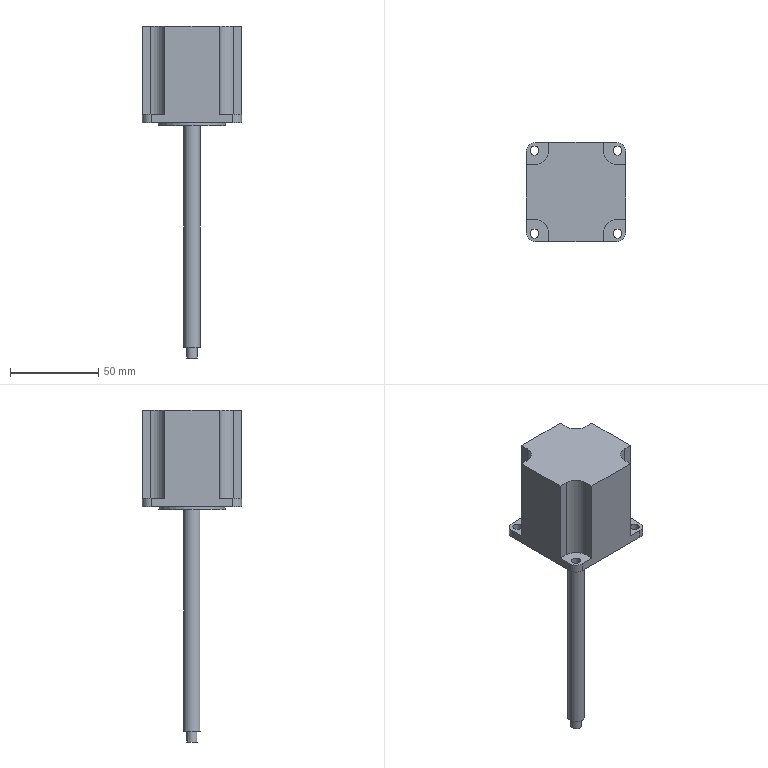Part | NX | features DATUM_CSYS 7, EXTRUDE 6, SKETCH 6, BLEND 1, DISTANCE MEASUREMENT 1, SYMBOLIC_THREAD 1 | 1 solid | 36 faces | box 56.4 x 56.4 x 188.6 mm | volume 156156 mm3 | plane 21 | cylinder 15 | commonest cylinder face diameters 5.1 x4 10 x4 16 x4 6 x1 9.525 x1 38.1 x1
STEP:
#1=CARTESIAN_POINT('',(-23.2,-28.2,4.8));
#2=VERTEX_POINT('',#1);
#3=CARTESIAN_POINT('',(-15.57,-28.2,4.8));
#4=VERTEX_POINT('',#3);
#5=CARTESIAN_POINT('',(-28.2,-28.2,4.8));
#6=DIRECTION('',(1.,0.,0.));
#7=VECTOR('',#6,1000.);
#8=LINE('',#5,#7);
#9=EDGE_CURVE('',#2,#4,#8,.T.);
#10=ORIENTED_EDGE('',*,*,#9,.F.);
#11=CARTESIAN_POINT('',(-23.2,-28.2,0.));
#12=VERTEX_POINT('',#11);
#13=CARTESIAN_POINT('',(-23.2,-28.2,55.));
#14=DIRECTION('',(0.,0.,-1.));
#15=VECTOR('',#14,1000.);
#16=LINE('',#13,#15);
#17=EDGE_CURVE('',#2,#12,#16,.T.);
#18=ORIENTED_EDGE('',*,*,#17,.T.);
#19=CARTESIAN_POINT('',(23.2,-28.2,0.));
#20=VERTEX_POINT('',#19);
#21=CARTESIAN_POINT('',(-28.2,-28.2,0.));
#22=DIRECTION('',(1.,0.,0.));
#23=VECTOR('',#22,1000.);
#24=LINE('',#21,#23);
#25=EDGE_CURVE('',#12,#20,#24,.T.);
#26=ORIENTED_EDGE('',*,*,#25,.T.);
#27=CARTESIAN_POINT('',(23.2,-28.2,4.8));
#28=VERTEX_POINT('',#27);
#29=CARTESIAN_POINT('',(23.2,-28.2,55.));
#30=DIRECTION('',(0.,0.,-1.));
#31=VECTOR('',#30,1000.);
#32=LINE('',#29,#31);
#33=EDGE_CURVE('',#20,#28,#32,.F.);
#34=ORIENTED_EDGE('',*,*,#33,.T.);
#35=CARTESIAN_POINT('',(15.57,-28.2,4.8));
#36=VERTEX_POINT('',#35);
#37=CARTESIAN_POINT('',(15.57,-28.2,4.8));
#38=DIRECTION('',(1.,0.,0.));
#39=VECTOR('',#38,1000.);
#40=LINE('',#37,#39);
#41=EDGE_CURVE('',#36,#28,#40,.T.);
#42=ORIENTED_EDGE('',*,*,#41,.F.);
#43=CARTESIAN_POINT('',(15.57,-28.2,55.));
#44=VERTEX_POINT('',#43);
#45=CARTESIAN_POINT('',(15.57,-28.2,4.8));
#46=DIRECTION('',(0.,0.,1.));
#47=VECTOR('',#46,1000.);
#48=LINE('',#45,#47);
#49=EDGE_CURVE('',#36,#44,#48,.T.);
#50=ORIENTED_EDGE('',*,*,#49,.T.);
#51=CARTESIAN_POINT('',(-15.57,-28.2,55.));
#52=VERTEX_POINT('',#51);
#53=CARTESIAN_POINT('',(-28.2,-28.2,55.));
#54=DIRECTION('',(1.,0.,0.));
#55=VECTOR('',#54,1000.);
#56=LINE('',#53,#55);
#57=EDGE_CURVE('',#52,#44,#56,.T.);
#58=ORIENTED_EDGE('',*,*,#57,.F.);
#59=CARTESIAN_POINT('',(-15.57,-28.2,4.8));
#60=DIRECTION('',(0.,0.,1.));
#61=VECTOR('',#60,1000.);
#62=LINE('',#59,#61);
#63=EDGE_CURVE('',#4,#52,#62,.T.);
#64=ORIENTED_EDGE('',*,*,#63,.F.);
#65=EDGE_LOOP('',(#10,#18,#26,#34,#42,#50,#58,#64));
#66=FACE_BOUND('',#65,.T.);
#67=CARTESIAN_POINT('',(-28.2,-28.2,55.));
#68=DIRECTION('',(0.,1.,0.));
#69=DIRECTION('',(0.,0.,1.));
#70=AXIS2_PLACEMENT_3D('',#67,#68,#69);
#71=PLANE('',#70);
#72=ADVANCED_FACE('',(#66),#71,.F.);
#73=CARTESIAN_POINT('',(-21.02,-23.57,0.));
#74=VERTEX_POINT('',#73);
#75=CARTESIAN_POINT('',(-23.57,-23.57,0.));
#76=DIRECTION('',(0.,0.,1.));
#77=DIRECTION('',(1.,0.,0.));
#78=AXIS2_PLACEMENT_3D('',#75,#76,#77);
#79=CIRCLE('',#78,2.55);
#80=EDGE_CURVE('',#74,#74,#79,.F.);
#81=ORIENTED_EDGE('',*,*,#80,.T.);
#82=EDGE_LOOP('',(#81));
#83=FACE_BOUND('',#82,.T.);
#84=CARTESIAN_POINT('',(-21.02,-23.57,4.8));
#85=VERTEX_POINT('',#84);
#86=CARTESIAN_POINT('',(-23.57,-23.57,4.8));
#87=DIRECTION('',(0.,0.,1.));
#88=DIRECTION('',(1.,0.,0.));
#89=AXIS2_PLACEMENT_3D('',#86,#87,#88);
#90=CIRCLE('',#89,2.55);
#91=EDGE_CURVE('',#85,#85,#90,.T.);
#92=ORIENTED_EDGE('',*,*,#91,.T.);
#93=EDGE_LOOP('',(#92));
#94=FACE_BOUND('',#93,.T.);
#95=CARTESIAN_POINT('',(-23.57,-23.57,-7.26));
#96=DIRECTION('',(0.,0.,1.));
#97=DIRECTION('',(1.,0.,0.));
#98=AXIS2_PLACEMENT_3D('',#95,#96,#97);
#99=CYLINDRICAL_SURFACE('',#98,2.55);
#100=ADVANCED_FACE('',(#83,#94),#99,.F.);
#101=CARTESIAN_POINT('',(-28.2,23.2,0.));
#102=VERTEX_POINT('',#101);
#103=CARTESIAN_POINT('',(-28.2,-23.2,0.));
#104=VERTEX_POINT('',#103);
#105=CARTESIAN_POINT('',(-28.2,28.2,0.));
#106=DIRECTION('',(0.,-1.,0.));
#107=VECTOR('',#106,1000.);
#108=LINE('',#105,#107);
#109=EDGE_CURVE('',#102,#104,#108,.T.);
#110=ORIENTED_EDGE('',*,*,#109,.T.);
#111=CARTESIAN_POINT('',(-28.2,-23.2,4.8));
#112=VERTEX_POINT('',#111);
#113=CARTESIAN_POINT('',(-28.2,-23.2,55.));
#114=DIRECTION('',(0.,0.,-1.));
#115=VECTOR('',#114,1000.);
#116=LINE('',#113,#115);
#117=EDGE_CURVE('',#104,#112,#116,.F.);
#118=ORIENTED_EDGE('',*,*,#117,.T.);
#119=CARTESIAN_POINT('',(-28.2,-15.57,4.8));
#120=VERTEX_POINT('',#119);
#121=CARTESIAN_POINT('',(-28.2,-15.57,4.8));
#122=DIRECTION('',(0.,-1.,0.));
#123=VECTOR('',#122,1000.);
#124=LINE('',#121,#123);
#125=EDGE_CURVE('',#120,#112,#124,.T.);
#126=ORIENTED_EDGE('',*,*,#125,.F.);
#127=CARTESIAN_POINT('',(-28.2,-15.57,55.));
#128=VERTEX_POINT('',#127);
#129=CARTESIAN_POINT('',(-28.2,-15.57,4.8));
#130=DIRECTION('',(0.,0.,1.));
#131=VECTOR('',#130,1000.);
#132=LINE('',#129,#131);
#133=EDGE_CURVE('',#120,#128,#132,.T.);
#134=ORIENTED_EDGE('',*,*,#133,.T.);
#135=CARTESIAN_POINT('',(-28.2,15.57,55.));
#136=VERTEX_POINT('',#135);
#137=CARTESIAN_POINT('',(-28.2,28.2,55.));
#138=DIRECTION('',(0.,-1.,0.));
#139=VECTOR('',#138,1000.);
#140=LINE('',#137,#139);
#141=EDGE_CURVE('',#136,#128,#140,.T.);
#142=ORIENTED_EDGE('',*,*,#141,.F.);
#143=CARTESIAN_POINT('',(-28.2,15.57,4.8));
#144=VERTEX_POINT('',#143);
#145=CARTESIAN_POINT('',(-28.2,15.57,4.8));
#146=DIRECTION('',(0.,0.,1.));
#147=VECTOR('',#146,1000.);
#148=LINE('',#145,#147);
#149=EDGE_CURVE('',#144,#136,#148,.T.);
#150=ORIENTED_EDGE('',*,*,#149,.F.);
#151=CARTESIAN_POINT('',(-28.2,23.2,4.8));
#152=VERTEX_POINT('',#151);
#153=CARTESIAN_POINT('',(-28.2,28.2,4.8));
#154=DIRECTION('',(0.,-1.,0.));
#155=VECTOR('',#154,1000.);
#156=LINE('',#153,#155);
#157=EDGE_CURVE('',#152,#144,#156,.T.);
#158=ORIENTED_EDGE('',*,*,#157,.F.);
#159=CARTESIAN_POINT('',(-28.2,23.2,55.));
#160=DIRECTION('',(0.,0.,-1.));
#161=VECTOR('',#160,1000.);
#162=LINE('',#159,#161);
#163=EDGE_CURVE('',#152,#102,#162,.T.);
#164=ORIENTED_EDGE('',*,*,#163,.T.);
#165=EDGE_LOOP('',(#110,#118,#126,#134,#142,#150,#158,#164));
#166=FACE_BOUND('',#165,.T.);
#167=CARTESIAN_POINT('',(-28.2,28.2,55.));
#168=DIRECTION('',(1.,0.,0.));
#169=DIRECTION('',(0.,0.,-1.));
#170=AXIS2_PLACEMENT_3D('',#167,#168,#169);
#171=PLANE('',#170);
#172=ADVANCED_FACE('',(#166),#171,.F.);
#173=CARTESIAN_POINT('',(28.2,-23.2,4.8));
#174=VERTEX_POINT('',#173);
#175=CARTESIAN_POINT('',(28.2,-15.57,4.8));
#176=VERTEX_POINT('',#175);
#177=CARTESIAN_POINT('',(28.2,-28.2,4.8));
#178=DIRECTION('',(0.,1.,0.));
#179=VECTOR('',#178,1000.);
#180=LINE('',#177,#179);
#181=EDGE_CURVE('',#174,#176,#180,.T.);
#182=ORIENTED_EDGE('',*,*,#181,.F.);
#183=CARTESIAN_POINT('',(28.2,-23.2,0.));
#184=VERTEX_POINT('',#183);
#185=CARTESIAN_POINT('',(28.2,-23.2,55.));
#186=DIRECTION('',(0.,0.,-1.));
#187=VECTOR('',#186,1000.);
#188=LINE('',#185,#187);
#189=EDGE_CURVE('',#174,#184,#188,.T.);
#190=ORIENTED_EDGE('',*,*,#189,.T.);
#191=CARTESIAN_POINT('',(28.2,23.2,0.));
#192=VERTEX_POINT('',#191);
#193=CARTESIAN_POINT('',(28.2,-28.2,0.));
#194=DIRECTION('',(0.,1.,0.));
#195=VECTOR('',#194,1000.);
#196=LINE('',#193,#195);
#197=EDGE_CURVE('',#184,#192,#196,.T.);
#198=ORIENTED_EDGE('',*,*,#197,.T.);
#199=CARTESIAN_POINT('',(28.2,23.2,4.8));
#200=VERTEX_POINT('',#199);
#201=CARTESIAN_POINT('',(28.2,23.2,55.));
#202=DIRECTION('',(0.,0.,-1.));
#203=VECTOR('',#202,1000.);
#204=LINE('',#201,#203);
#205=EDGE_CURVE('',#192,#200,#204,.F.);
#206=ORIENTED_EDGE('',*,*,#205,.T.);
#207=CARTESIAN_POINT('',(28.2,15.57,4.8));
#208=VERTEX_POINT('',#207);
#209=CARTESIAN_POINT('',(28.2,15.57,4.8));
#210=DIRECTION('',(0.,1.,0.));
#211=VECTOR('',#210,1000.);
#212=LINE('',#209,#211);
#213=EDGE_CURVE('',#208,#200,#212,.T.);
#214=ORIENTED_EDGE('',*,*,#213,.F.);
#215=CARTESIAN_POINT('',(28.2,15.57,55.));
#216=VERTEX_POINT('',#215);
#217=CARTESIAN_POINT('',(28.2,15.57,4.8));
#218=DIRECTION('',(0.,0.,1.));
#219=VECTOR('',#218,1000.);
#220=LINE('',#217,#219);
#221=EDGE_CURVE('',#208,#216,#220,.T.);
#222=ORIENTED_EDGE('',*,*,#221,.T.);
#223=CARTESIAN_POINT('',(28.2,-15.57,55.));
#224=VERTEX_POINT('',#223);
#225=CARTESIAN_POINT('',(28.2,-28.2,55.));
#226=DIRECTION('',(0.,1.,0.));
#227=VECTOR('',#226,1000.);
#228=LINE('',#225,#227);
#229=EDGE_CURVE('',#224,#216,#228,.T.);
#230=ORIENTED_EDGE('',*,*,#229,.F.);
#231=CARTESIAN_POINT('',(28.2,-15.57,4.8));
#232=DIRECTION('',(0.,0.,1.));
#233=VECTOR('',#232,1000.);
#234=LINE('',#231,#233);
#235=EDGE_CURVE('',#176,#224,#234,.T.);
#236=ORIENTED_EDGE('',*,*,#235,.F.);
#237=EDGE_LOOP('',(#182,#190,#198,#206,#214,#222,#230,#236));
#238=FACE_BOUND('',#237,.T.);
#239=CARTESIAN_POINT('',(28.2,-28.2,55.));
#240=DIRECTION('',(-1.,0.,0.));
#241=DIRECTION('',(0.,0.,1.));
#242=AXIS2_PLACEMENT_3D('',#239,#240,#241);
#243=PLANE('',#242);
#244=ADVANCED_FACE('',(#238),#243,.F.);
#245=CARTESIAN_POINT('',(23.2,28.2,4.8));
#246=VERTEX_POINT('',#245);
#247=CARTESIAN_POINT('',(15.57,28.2,4.8));
#248=VERTEX_POINT('',#247);
#249=CARTESIAN_POINT('',(28.2,28.2,4.8));
#250=DIRECTION('',(-1.,0.,0.));
#251=VECTOR('',#250,1000.);
#252=LINE('',#249,#251);
#253=EDGE_CURVE('',#246,#248,#252,.T.);
#254=ORIENTED_EDGE('',*,*,#253,.F.);
#255=CARTESIAN_POINT('',(23.2,28.2,0.));
#256=VERTEX_POINT('',#255);
#257=CARTESIAN_POINT('',(23.2,28.2,55.));
#258=DIRECTION('',(0.,0.,-1.));
#259=VECTOR('',#258,1000.);
#260=LINE('',#257,#259);
#261=EDGE_CURVE('',#246,#256,#260,.T.);
#262=ORIENTED_EDGE('',*,*,#261,.T.);
#263=CARTESIAN_POINT('',(-23.2,28.2,0.));
#264=VERTEX_POINT('',#263);
#265=CARTESIAN_POINT('',(28.2,28.2,0.));
#266=DIRECTION('',(-1.,0.,0.));
#267=VECTOR('',#266,1000.);
#268=LINE('',#265,#267);
#269=EDGE_CURVE('',#256,#264,#268,.T.);
#270=ORIENTED_EDGE('',*,*,#269,.T.);
#271=CARTESIAN_POINT('',(-23.2,28.2,4.8));
#272=VERTEX_POINT('',#271);
#273=CARTESIAN_POINT('',(-23.2,28.2,55.));
#274=DIRECTION('',(0.,0.,-1.));
#275=VECTOR('',#274,1000.);
#276=LINE('',#273,#275);
#277=EDGE_CURVE('',#264,#272,#276,.F.);
#278=ORIENTED_EDGE('',*,*,#277,.T.);
#279=CARTESIAN_POINT('',(-15.57,28.2,4.8));
#280=VERTEX_POINT('',#279);
#281=CARTESIAN_POINT('',(-15.57,28.2,4.8));
#282=DIRECTION('',(-1.,0.,0.));
#283=VECTOR('',#282,1000.);
#284=LINE('',#281,#283);
#285=EDGE_CURVE('',#280,#272,#284,.T.);
#286=ORIENTED_EDGE('',*,*,#285,.F.);
#287=CARTESIAN_POINT('',(-15.57,28.2,55.));
#288=VERTEX_POINT('',#287);
#289=CARTESIAN_POINT('',(-15.57,28.2,4.8));
#290=DIRECTION('',(0.,0.,1.));
#291=VECTOR('',#290,1000.);
#292=LINE('',#289,#291);
#293=EDGE_CURVE('',#280,#288,#292,.T.);
#294=ORIENTED_EDGE('',*,*,#293,.T.);
#295=CARTESIAN_POINT('',(15.57,28.2,55.));
#296=VERTEX_POINT('',#295);
#297=CARTESIAN_POINT('',(28.2,28.2,55.));
#298=DIRECTION('',(-1.,0.,0.));
#299=VECTOR('',#298,1000.);
#300=LINE('',#297,#299);
#301=EDGE_CURVE('',#296,#288,#300,.T.);
#302=ORIENTED_EDGE('',*,*,#301,.F.);
#303=CARTESIAN_POINT('',(15.57,28.2,4.8));
#304=DIRECTION('',(0.,0.,1.));
#305=VECTOR('',#304,1000.);
#306=LINE('',#303,#305);
#307=EDGE_CURVE('',#248,#296,#306,.T.);
#308=ORIENTED_EDGE('',*,*,#307,.F.);
#309=EDGE_LOOP('',(#254,#262,#270,#278,#286,#294,#302,#308));
#310=FACE_BOUND('',#309,.T.);
#311=CARTESIAN_POINT('',(28.2,28.2,55.));
#312=DIRECTION('',(0.,-1.,0.));
#313=DIRECTION('',(1.,0.,0.));
#314=AXIS2_PLACEMENT_3D('',#311,#312,#313);
#315=PLANE('',#314);
#316=ADVANCED_FACE('',(#310),#315,.F.);
#317=CARTESIAN_POINT('',(-15.57,-23.57,55.));
#318=VERTEX_POINT('',#317);
#319=CARTESIAN_POINT('',(-15.57,-28.2,55.));
#320=DIRECTION('',(0.,1.,0.));
#321=VECTOR('',#320,1000.);
#322=LINE('',#319,#321);
#323=EDGE_CURVE('',#52,#318,#322,.T.);
#324=ORIENTED_EDGE('',*,*,#323,.F.);
#325=ORIENTED_EDGE('',*,*,#57,.T.);
#326=CARTESIAN_POINT('',(15.57,-23.57,55.));
#327=VERTEX_POINT('',#326);
#328=CARTESIAN_POINT('',(15.57,-23.57,55.));
#329=DIRECTION('',(0.,-1.,0.));
#330=VECTOR('',#329,1000.);
#331=LINE('',#328,#330);
#332=EDGE_CURVE('',#327,#44,#331,.T.);
#333=ORIENTED_EDGE('',*,*,#332,.F.);
#334=CARTESIAN_POINT('',(23.57,-15.57,55.));
#335=VERTEX_POINT('',#334);
#336=CARTESIAN_POINT('',(23.57,-23.57,55.));
#337=DIRECTION('',(0.,0.,1.));
#338=DIRECTION('',(0.,1.,0.));
#339=AXIS2_PLACEMENT_3D('',#336,#337,#338);
#340=CIRCLE('',#339,8.);
#341=EDGE_CURVE('',#335,#327,#340,.T.);
#342=ORIENTED_EDGE('',*,*,#341,.F.);
#343=CARTESIAN_POINT('',(28.2,-15.57,55.));
#344=DIRECTION('',(-1.,0.,0.));
#345=VECTOR('',#344,1000.);
#346=LINE('',#343,#345);
#347=EDGE_CURVE('',#224,#335,#346,.T.);
#348=ORIENTED_EDGE('',*,*,#347,.F.);
#349=ORIENTED_EDGE('',*,*,#229,.T.);
#350=CARTESIAN_POINT('',(23.57,15.57,55.));
#351=VERTEX_POINT('',#350);
#352=CARTESIAN_POINT('',(23.57,15.57,55.));
#353=DIRECTION('',(1.,0.,0.));
#354=VECTOR('',#353,1000.);
#355=LINE('',#352,#354);
#356=EDGE_CURVE('',#351,#216,#355,.T.);
#357=ORIENTED_EDGE('',*,*,#356,.F.);
#358=CARTESIAN_POINT('',(15.57,23.57,55.));
#359=VERTEX_POINT('',#358);
#360=CARTESIAN_POINT('',(23.57,23.57,55.));
#361=DIRECTION('',(0.,0.,1.));
#362=DIRECTION('',(0.,-1.,0.));
#363=AXIS2_PLACEMENT_3D('',#360,#361,#362);
#364=CIRCLE('',#363,8.);
#365=EDGE_CURVE('',#359,#351,#364,.T.);
#366=ORIENTED_EDGE('',*,*,#365,.F.);
#367=CARTESIAN_POINT('',(15.57,28.2,55.));
#368=DIRECTION('',(0.,-1.,0.));
#369=VECTOR('',#368,1000.);
#370=LINE('',#367,#369);
#371=EDGE_CURVE('',#296,#359,#370,.T.);
#372=ORIENTED_EDGE('',*,*,#371,.F.);
#373=ORIENTED_EDGE('',*,*,#301,.T.);
#374=CARTESIAN_POINT('',(-15.57,23.57,55.));
#375=VERTEX_POINT('',#374);
#376=CARTESIAN_POINT('',(-15.57,23.57,55.));
#377=DIRECTION('',(0.,1.,0.));
#378=VECTOR('',#377,1000.);
#379=LINE('',#376,#378);
#380=EDGE_CURVE('',#375,#288,#379,.T.);
#381=ORIENTED_EDGE('',*,*,#380,.F.);
#382=CARTESIAN_POINT('',(-23.57,15.57,55.));
#383=VERTEX_POINT('',#382);
#384=CARTESIAN_POINT('',(-23.57,23.57,55.));
#385=DIRECTION('',(0.,0.,1.));
#386=DIRECTION('',(0.,-1.,0.));
#387=AXIS2_PLACEMENT_3D('',#384,#385,#386);
#388=CIRCLE('',#387,8.);
#389=EDGE_CURVE('',#383,#375,#388,.T.);
#390=ORIENTED_EDGE('',*,*,#389,.F.);
#391=CARTESIAN_POINT('',(-28.2,15.57,55.));
#392=DIRECTION('',(1.,0.,0.));
#393=VECTOR('',#392,1000.);
#394=LINE('',#391,#393);
#395=EDGE_CURVE('',#136,#383,#394,.T.);
#396=ORIENTED_EDGE('',*,*,#395,.F.);
#397=ORIENTED_EDGE('',*,*,#141,.T.);
#398=CARTESIAN_POINT('',(-23.57,-15.57,55.));
#399=VERTEX_POINT('',#398);
#400=CARTESIAN_POINT('',(-23.57,-15.57,55.));
#401=DIRECTION('',(-1.,0.,0.));
#402=VECTOR('',#401,1000.);
#403=LINE('',#400,#402);
#404=EDGE_CURVE('',#399,#128,#403,.T.);
#405=ORIENTED_EDGE('',*,*,#404,.F.);
#406=CARTESIAN_POINT('',(-23.57,-23.57,55.));
#407=DIRECTION('',(0.,0.,1.));
#408=DIRECTION('',(0.,1.,0.));
#409=AXIS2_PLACEMENT_3D('',#406,#407,#408);
#410=CIRCLE('',#409,8.);
#411=EDGE_CURVE('',#318,#399,#410,.T.);
#412=ORIENTED_EDGE('',*,*,#411,.F.);
#413=EDGE_LOOP('',(#324,#325,#333,#342,#348,#349,#357,#366,#372,#373,#381,#390,#396,#397,#405,#412));
#414=FACE_BOUND('',#413,.T.);
#415=CARTESIAN_POINT('',(0.,0.,55.));
#416=DIRECTION('',(0.,0.,1.));
#417=DIRECTION('',(1.,0.,0.));
#418=AXIS2_PLACEMENT_3D('',#415,#416,#417);
#419=PLANE('',#418);
#420=ADVANCED_FACE('',(#414),#419,.T.);
#421=CARTESIAN_POINT('',(26.12,23.57,0.));
#422=VERTEX_POINT('',#421);
#423=CARTESIAN_POINT('',(23.57,23.57,0.));
#424=DIRECTION('',(0.,0.,1.));
#425=DIRECTION('',(1.,0.,0.));
#426=AXIS2_PLACEMENT_3D('',#423,#424,#425);
#427=CIRCLE('',#426,2.55);
#428=EDGE_CURVE('',#422,#422,#427,.F.);
#429=ORIENTED_EDGE('',*,*,#428,.F.);
#430=EDGE_LOOP('',(#429));
#431=FACE_BOUND('',#430,.T.);
#432=CARTESIAN_POINT('',(26.12,-23.57,0.));
#433=VERTEX_POINT('',#432);
#434=CARTESIAN_POINT('',(23.57,-23.57,0.));
#435=DIRECTION('',(0.,0.,1.));
#436=DIRECTION('',(1.,0.,0.));
#437=AXIS2_PLACEMENT_3D('',#434,#435,#436);
#438=CIRCLE('',#437,2.55);
#439=EDGE_CURVE('',#433,#433,#438,.T.);
#440=ORIENTED_EDGE('',*,*,#439,.T.);
#441=EDGE_LOOP('',(#440));
#442=FACE_BOUND('',#441,.T.);
#443=CARTESIAN_POINT('',(-21.02,23.57,0.));
#444=VERTEX_POINT('',#443);
#445=CARTESIAN_POINT('',(-23.57,23.57,0.));
#446=DIRECTION('',(0.,0.,1.));
#447=DIRECTION('',(1.,0.,0.));
#448=AXIS2_PLACEMENT_3D('',#445,#446,#447);
#449=CIRCLE('',#448,2.55);
#450=EDGE_CURVE('',#444,#444,#449,.T.);
#451=ORIENTED_EDGE('',*,*,#450,.T.);
#452=EDGE_LOOP('',(#451));
#453=FACE_BOUND('',#452,.T.);
#454=ORIENTED_EDGE('',*,*,#80,.F.);
#455=EDGE_LOOP('',(#454));
#456=FACE_BOUND('',#455,.T.);
#457=CARTESIAN_POINT('',(19.05,0.,0.));
#458=VERTEX_POINT('',#457);
#459=CARTESIAN_POINT('',(0.,0.,0.));
#460=DIRECTION('',(0.,0.,1.));
#461=DIRECTION('',(1.,0.,0.));
#462=AXIS2_PLACEMENT_3D('',#459,#460,#461);
#463=CIRCLE('',#462,19.05);
#464=EDGE_CURVE('',#458,#458,#463,.F.);
#465=ORIENTED_EDGE('',*,*,#464,.F.);
#466=EDGE_LOOP('',(#465));
#467=FACE_BOUND('',#466,.T.);
#468=ORIENTED_EDGE('',*,*,#25,.F.);
#469=CARTESIAN_POINT('',(-23.2,-23.2,0.));
#470=DIRECTION('',(0.,0.,1.));
#471=DIRECTION('',(1.,0.,0.));
#472=AXIS2_PLACEMENT_3D('',#469,#470,#471);
#473=CIRCLE('',#472,5.);
#474=EDGE_CURVE('',#12,#104,#473,.F.);
#475=ORIENTED_EDGE('',*,*,#474,.T.);
#476=ORIENTED_EDGE('',*,*,#109,.F.);
#477=CARTESIAN_POINT('',(-23.2,23.2,0.));
#478=DIRECTION('',(0.,0.,1.));
#479=DIRECTION('',(1.,0.,0.));
#480=AXIS2_PLACEMENT_3D('',#477,#478,#479);
#481=CIRCLE('',#480,5.);
#482=EDGE_CURVE('',#102,#264,#481,.F.);
#483=ORIENTED_EDGE('',*,*,#482,.T.);
#484=ORIENTED_EDGE('',*,*,#269,.F.);
#485=CARTESIAN_POINT('',(23.2,23.2,0.));
#486=DIRECTION('',(0.,0.,1.));
#487=DIRECTION('',(1.,0.,0.));
#488=AXIS2_PLACEMENT_3D('',#485,#486,#487);
#489=CIRCLE('',#488,5.);
#490=EDGE_CURVE('',#256,#192,#489,.F.);
#491=ORIENTED_EDGE('',*,*,#490,.T.);
#492=ORIENTED_EDGE('',*,*,#197,.F.);
#493=CARTESIAN_POINT('',(23.2,-23.2,0.));
#494=DIRECTION('',(0.,0.,1.));
#495=DIRECTION('',(1.,0.,0.));
#496=AXIS2_PLACEMENT_3D('',#493,#494,#495);
#497=CIRCLE('',#496,5.);
#498=EDGE_CURVE('',#184,#20,#497,.F.);
#499=ORIENTED_EDGE('',*,*,#498,.T.);
#500=EDGE_LOOP('',(#468,#475,#476,#483,#484,#491,#492,#499));
#501=FACE_BOUND('',#500,.T.);
#502=CARTESIAN_POINT('',(0.,0.,0.));
#503=DIRECTION('',(0.,0.,1.));
#504=DIRECTION('',(1.,0.,0.));
#505=AXIS2_PLACEMENT_3D('',#502,#503,#504);
#506=PLANE('',#505);
#507=ADVANCED_FACE('',(#431,#442,#453,#456,#467,#501),#506,.F.);
#508=CARTESIAN_POINT('',(19.05,0.,-1.6));
#509=VERTEX_POINT('',#508);
#510=CARTESIAN_POINT('',(0.,0.,-1.6));
#511=DIRECTION('',(0.,0.,1.));
#512=DIRECTION('',(1.,0.,0.));
#513=AXIS2_PLACEMENT_3D('',#510,#511,#512);
#514=CIRCLE('',#513,19.05);
#515=EDGE_CURVE('',#509,#509,#514,.F.);
#516=ORIENTED_EDGE('',*,*,#515,.F.);
#517=EDGE_LOOP('',(#516));
#518=FACE_BOUND('',#517,.T.);
#519=ORIENTED_EDGE('',*,*,#464,.T.);
#520=EDGE_LOOP('',(#519));
#521=FACE_BOUND('',#520,.T.);
#522=CARTESIAN_POINT('',(0.,0.,-1.6));
#523=DIRECTION('',(0.,0.,1.));
#524=DIRECTION('',(1.,0.,0.));
#525=AXIS2_PLACEMENT_3D('',#522,#523,#524);
#526=CYLINDRICAL_SURFACE('',#525,19.05);
#527=ADVANCED_FACE('',(#518,#521),#526,.T.);
#528=CARTESIAN_POINT('',(4.763,0.,-1.6));
#529=VERTEX_POINT('',#528);
#530=CARTESIAN_POINT('',(0.,0.,-1.6));
#531=DIRECTION('',(0.,0.,-1.));
#532=DIRECTION('',(1.,0.,0.));
#533=AXIS2_PLACEMENT_3D('',#530,#531,#532);
#534=CIRCLE('',#533,4.763);
#535=EDGE_CURVE('',#529,#529,#534,.T.);
#536=ORIENTED_EDGE('',*,*,#535,.F.);
#537=EDGE_LOOP('',(#536));
#538=FACE_BOUND('',#537,.T.);
#539=ORIENTED_EDGE('',*,*,#515,.T.);
#540=EDGE_LOOP('',(#539));
#541=FACE_BOUND('',#540,.T.);
#542=CARTESIAN_POINT('',(0.,0.,-1.6));
#543=DIRECTION('',(0.,0.,1.));
#544=DIRECTION('',(1.,0.,0.));
#545=AXIS2_PLACEMENT_3D('',#542,#543,#544);
#546=PLANE('',#545);
#547=ADVANCED_FACE('',(#538,#541),#546,.F.);
#548=CARTESIAN_POINT('',(-21.02,23.57,4.8));
#549=VERTEX_POINT('',#548);
#550=CARTESIAN_POINT('',(-23.57,23.57,4.8));
#551=DIRECTION('',(0.,0.,1.));
#552=DIRECTION('',(1.,0.,0.));
#553=AXIS2_PLACEMENT_3D('',#550,#551,#552);
#554=CIRCLE('',#553,2.55);
#555=EDGE_CURVE('',#549,#549,#554,.T.);
#556=ORIENTED_EDGE('',*,*,#555,.T.);
#557=EDGE_LOOP('',(#556));
#558=FACE_BOUND('',#557,.T.);
#559=ORIENTED_EDGE('',*,*,#450,.F.);
#560=EDGE_LOOP('',(#559));
#561=FACE_BOUND('',#560,.T.);
#562=CARTESIAN_POINT('',(-23.57,23.57,-7.26));
#563=DIRECTION('',(0.,0.,1.));
#564=DIRECTION('',(1.,0.,0.));
#565=AXIS2_PLACEMENT_3D('',#562,#563,#564);
#566=CYLINDRICAL_SURFACE('',#565,2.55);
#567=ADVANCED_FACE('',(#558,#561),#566,.F.);
#568=CARTESIAN_POINT('',(21.02,-23.57,4.8));
#569=VERTEX_POINT('',#568);
#570=CARTESIAN_POINT('',(23.57,-23.57,4.8));
#571=DIRECTION('',(0.,0.,1.));
#572=DIRECTION('',(-1.,0.,0.));
#573=AXIS2_PLACEMENT_3D('',#570,#571,#572);
#574=CIRCLE('',#573,2.55);
#575=EDGE_CURVE('',#569,#569,#574,.T.);
#576=ORIENTED_EDGE('',*,*,#575,.T.);
#577=EDGE_LOOP('',(#576));
#578=FACE_BOUND('',#577,.T.);
#579=ORIENTED_EDGE('',*,*,#439,.F.);
#580=EDGE_LOOP('',(#579));
#581=FACE_BOUND('',#580,.T.);
#582=CARTESIAN_POINT('',(23.57,-23.57,-7.26));
#583=DIRECTION('',(0.,0.,1.));
#584=DIRECTION('',(1.,0.,0.));
#585=AXIS2_PLACEMENT_3D('',#582,#583,#584);
#586=CYLINDRICAL_SURFACE('',#585,2.55);
#587=ADVANCED_FACE('',(#578,#581),#586,.F.);
#588=CARTESIAN_POINT('',(21.02,23.57,4.8));
#589=VERTEX_POINT('',#588);
#590=CARTESIAN_POINT('',(23.57,23.57,4.8));
#591=DIRECTION('',(0.,0.,-1.));
#592=DIRECTION('',(-1.,0.,0.));
#593=AXIS2_PLACEMENT_3D('',#590,#591,#592);
#594=CIRCLE('',#593,2.55);
#595=EDGE_CURVE('',#589,#589,#594,.T.);
#596=ORIENTED_EDGE('',*,*,#595,.F.);
#597=EDGE_LOOP('',(#596));
#598=FACE_BOUND('',#597,.T.);
#599=ORIENTED_EDGE('',*,*,#428,.T.);
#600=EDGE_LOOP('',(#599));
#601=FACE_BOUND('',#600,.T.);
#602=CARTESIAN_POINT('',(23.57,23.57,-7.26));
#603=DIRECTION('',(0.,0.,1.));
#604=DIRECTION('',(1.,0.,0.));
#605=AXIS2_PLACEMENT_3D('',#602,#603,#604);
#606=CYLINDRICAL_SURFACE('',#605,2.55);
#607=ADVANCED_FACE('',(#598,#601),#606,.F.);
#608=ORIENTED_EDGE('',*,*,#371,.T.);
#609=CARTESIAN_POINT('',(15.57,23.57,4.8));
#610=VERTEX_POINT('',#609);
#611=CARTESIAN_POINT('',(15.57,23.57,4.8));
#612=DIRECTION('',(0.,0.,1.));
#613=VECTOR('',#612,1000.);
#614=LINE('',#611,#613);
#615=EDGE_CURVE('',#359,#610,#614,.F.);
#616=ORIENTED_EDGE('',*,*,#615,.T.);
#617=CARTESIAN_POINT('',(15.57,28.2,4.8));
#618=DIRECTION('',(0.,-1.,0.));
#619=VECTOR('',#618,1000.);
#620=LINE('',#617,#619);
#621=EDGE_CURVE('',#610,#248,#620,.F.);
#622=ORIENTED_EDGE('',*,*,#621,.T.);
#623=ORIENTED_EDGE('',*,*,#307,.T.);
#624=EDGE_LOOP('',(#608,#616,#622,#623));
#625=FACE_BOUND('',#624,.T.);
#626=CARTESIAN_POINT('',(15.57,28.2,4.8));
#627=DIRECTION('',(-1.,0.,0.));
#628=DIRECTION('',(0.,0.,1.));
#629=AXIS2_PLACEMENT_3D('',#626,#627,#628);
#630=PLANE('',#629);
#631=ADVANCED_FACE('',(#625),#630,.F.);
#632=ORIENTED_EDGE('',*,*,#365,.T.);
#633=CARTESIAN_POINT('',(23.57,15.57,4.8));
#634=VERTEX_POINT('',#633);
#635=CARTESIAN_POINT('',(23.57,15.57,4.8));
#636=DIRECTION('',(0.,0.,1.));
#637=VECTOR('',#636,1000.);
#638=LINE('',#635,#637);
#639=EDGE_CURVE('',#351,#634,#638,.F.);
#640=ORIENTED_EDGE('',*,*,#639,.T.);
#641=CARTESIAN_POINT('',(23.57,23.57,4.8));
#642=DIRECTION('',(0.,0.,1.));
#643=DIRECTION('',(0.,-1.,0.));
#644=AXIS2_PLACEMENT_3D('',#641,#642,#643);
#645=CIRCLE('',#644,8.);
#646=EDGE_CURVE('',#634,#610,#645,.F.);
#647=ORIENTED_EDGE('',*,*,#646,.T.);
#648=ORIENTED_EDGE('',*,*,#615,.F.);
#649=EDGE_LOOP('',(#632,#640,#647,#648));
#650=FACE_BOUND('',#649,.T.);
#651=CARTESIAN_POINT('',(23.57,23.57,4.8));
#652=DIRECTION('',(0.,0.,1.));
#653=DIRECTION('',(1.,0.,0.));
#654=AXIS2_PLACEMENT_3D('',#651,#652,#653);
#655=CYLINDRICAL_SURFACE('',#654,8.);
#656=ADVANCED_FACE('',(#650),#655,.F.);
#657=ORIENTED_EDGE('',*,*,#356,.T.);
#658=ORIENTED_EDGE('',*,*,#221,.F.);
#659=CARTESIAN_POINT('',(23.57,15.57,4.8));
#660=DIRECTION('',(1.,0.,0.));
#661=VECTOR('',#660,1000.);
#662=LINE('',#659,#661);
#663=EDGE_CURVE('',#208,#634,#662,.F.);
#664=ORIENTED_EDGE('',*,*,#663,.T.);
#665=ORIENTED_EDGE('',*,*,#639,.F.);
#666=EDGE_LOOP('',(#657,#658,#664,#665));
#667=FACE_BOUND('',#666,.T.);
#668=CARTESIAN_POINT('',(23.57,15.57,4.8));
#669=DIRECTION('',(0.,-1.,0.));
#670=DIRECTION('',(0.,0.,-1.));
#671=AXIS2_PLACEMENT_3D('',#668,#669,#670);
#672=PLANE('',#671);
#673=ADVANCED_FACE('',(#667),#672,.F.);
#674=ORIENTED_EDGE('',*,*,#213,.T.);
#675=CARTESIAN_POINT('',(23.2,23.2,4.8));
#676=DIRECTION('',(0.,0.,1.));
#677=DIRECTION('',(1.,0.,0.));
#678=AXIS2_PLACEMENT_3D('',#675,#676,#677);
#679=CIRCLE('',#678,5.);
#680=EDGE_CURVE('',#200,#246,#679,.T.);
#681=ORIENTED_EDGE('',*,*,#680,.T.);
#682=ORIENTED_EDGE('',*,*,#253,.T.);
#683=ORIENTED_EDGE('',*,*,#621,.F.);
#684=ORIENTED_EDGE('',*,*,#646,.F.);
#685=ORIENTED_EDGE('',*,*,#663,.F.);
#686=EDGE_LOOP('',(#674,#681,#682,#683,#684,#685));
#687=FACE_BOUND('',#686,.T.);
#688=ORIENTED_EDGE('',*,*,#595,.T.);
#689=EDGE_LOOP('',(#688));
#690=FACE_BOUND('',#689,.T.);
#691=CARTESIAN_POINT('',(23.57,23.57,4.8));
#692=DIRECTION('',(0.,0.,1.));
#693=DIRECTION('',(1.,0.,0.));
#694=AXIS2_PLACEMENT_3D('',#691,#692,#693);
#695=PLANE('',#694);
#696=ADVANCED_FACE('',(#687,#690),#695,.T.);
#697=ORIENTED_EDGE('',*,*,#332,.T.);
#698=ORIENTED_EDGE('',*,*,#49,.F.);
#699=CARTESIAN_POINT('',(15.57,-23.57,4.8));
#700=VERTEX_POINT('',#699);
#701=CARTESIAN_POINT('',(15.57,-23.57,4.8));
#702=DIRECTION('',(0.,-1.,0.));
#703=VECTOR('',#702,1000.);
#704=LINE('',#701,#703);
#705=EDGE_CURVE('',#36,#700,#704,.F.);
#706=ORIENTED_EDGE('',*,*,#705,.T.);
#707=CARTESIAN_POINT('',(15.57,-23.57,4.8));
#708=DIRECTION('',(0.,0.,1.));
#709=VECTOR('',#708,1000.);
#710=LINE('',#707,#709);
#711=EDGE_CURVE('',#327,#700,#710,.F.);
#712=ORIENTED_EDGE('',*,*,#711,.F.);
#713=EDGE_LOOP('',(#697,#698,#706,#712));
#714=FACE_BOUND('',#713,.T.);
#715=CARTESIAN_POINT('',(15.57,-23.57,4.8));
#716=DIRECTION('',(-1.,0.,0.));
#717=DIRECTION('',(0.,0.,1.));
#718=AXIS2_PLACEMENT_3D('',#715,#716,#717);
#719=PLANE('',#718);
#720=ADVANCED_FACE('',(#714),#719,.F.);
#721=ORIENTED_EDGE('',*,*,#347,.T.);
#722=CARTESIAN_POINT('',(23.57,-15.57,4.8));
#723=VERTEX_POINT('',#722);
#724=CARTESIAN_POINT('',(23.57,-15.57,4.8));
#725=DIRECTION('',(0.,0.,1.));
#726=VECTOR('',#725,1000.);
#727=LINE('',#724,#726);
#728=EDGE_CURVE('',#335,#723,#727,.F.);
#729=ORIENTED_EDGE('',*,*,#728,.T.);
#730=CARTESIAN_POINT('',(28.2,-15.57,4.8));
#731=DIRECTION('',(-1.,0.,0.));
#732=VECTOR('',#731,1000.);
#733=LINE('',#730,#732);
#734=EDGE_CURVE('',#723,#176,#733,.F.);
#735=ORIENTED_EDGE('',*,*,#734,.T.);
#736=ORIENTED_EDGE('',*,*,#235,.T.);
#737=EDGE_LOOP('',(#721,#729,#735,#736));
#738=FACE_BOUND('',#737,.T.);
#739=CARTESIAN_POINT('',(28.2,-15.57,4.8));
#740=DIRECTION('',(0.,1.,0.));
#741=DIRECTION('',(0.,0.,1.));
#742=AXIS2_PLACEMENT_3D('',#739,#740,#741);
#743=PLANE('',#742);
#744=ADVANCED_FACE('',(#738),#743,.F.);
#745=ORIENTED_EDGE('',*,*,#341,.T.);
#746=ORIENTED_EDGE('',*,*,#711,.T.);
#747=CARTESIAN_POINT('',(23.57,-23.57,4.8));
#748=DIRECTION('',(0.,0.,1.));
#749=DIRECTION('',(0.,1.,0.));
#750=AXIS2_PLACEMENT_3D('',#747,#748,#749);
#751=CIRCLE('',#750,8.);
#752=EDGE_CURVE('',#700,#723,#751,.F.);
#753=ORIENTED_EDGE('',*,*,#752,.T.);
#754=ORIENTED_EDGE('',*,*,#728,.F.);
#755=EDGE_LOOP('',(#745,#746,#753,#754));
#756=FACE_BOUND('',#755,.T.);
#757=CARTESIAN_POINT('',(23.57,-23.57,4.8));
#758=DIRECTION('',(0.,0.,1.));
#759=DIRECTION('',(1.,0.,0.));
#760=AXIS2_PLACEMENT_3D('',#757,#758,#759);
#761=CYLINDRICAL_SURFACE('',#760,8.);
#762=ADVANCED_FACE('',(#756),#761,.F.);
#763=ORIENTED_EDGE('',*,*,#41,.T.);
#764=CARTESIAN_POINT('',(23.2,-23.2,4.8));
#765=DIRECTION('',(0.,0.,1.));
#766=DIRECTION('',(1.,0.,0.));
#767=AXIS2_PLACEMENT_3D('',#764,#765,#766);
#768=CIRCLE('',#767,5.);
#769=EDGE_CURVE('',#28,#174,#768,.T.);
#770=ORIENTED_EDGE('',*,*,#769,.T.);
#771=ORIENTED_EDGE('',*,*,#181,.T.);
#772=ORIENTED_EDGE('',*,*,#734,.F.);
#773=ORIENTED_EDGE('',*,*,#752,.F.);
#774=ORIENTED_EDGE('',*,*,#705,.F.);
#775=EDGE_LOOP('',(#763,#770,#771,#772,#773,#774));
#776=FACE_BOUND('',#775,.T.);
#777=ORIENTED_EDGE('',*,*,#575,.F.);
#778=EDGE_LOOP('',(#777));
#779=FACE_BOUND('',#778,.T.);
#780=CARTESIAN_POINT('',(23.57,-23.57,4.8));
#781=DIRECTION('',(0.,0.,1.));
#782=DIRECTION('',(1.,0.,0.));
#783=AXIS2_PLACEMENT_3D('',#780,#781,#782);
#784=PLANE('',#783);
#785=ADVANCED_FACE('',(#776,#779),#784,.T.);
#786=ORIENTED_EDGE('',*,*,#395,.T.);
#787=CARTESIAN_POINT('',(-23.57,15.57,4.8));
#788=VERTEX_POINT('',#787);
#789=CARTESIAN_POINT('',(-23.57,15.57,4.8));
#790=DIRECTION('',(0.,0.,1.));
#791=VECTOR('',#790,1000.);
#792=LINE('',#789,#791);
#793=EDGE_CURVE('',#383,#788,#792,.F.);
#794=ORIENTED_EDGE('',*,*,#793,.T.);
#795=CARTESIAN_POINT('',(-28.2,15.57,4.8));
#796=DIRECTION('',(1.,0.,0.));
#797=VECTOR('',#796,1000.);
#798=LINE('',#795,#797);
#799=EDGE_CURVE('',#788,#144,#798,.F.);
#800=ORIENTED_EDGE('',*,*,#799,.T.);
#801=ORIENTED_EDGE('',*,*,#149,.T.);
#802=EDGE_LOOP('',(#786,#794,#800,#801));
#803=FACE_BOUND('',#802,.T.);
#804=CARTESIAN_POINT('',(-28.2,15.57,4.8));
#805=DIRECTION('',(0.,-1.,0.));
#806=DIRECTION('',(0.,0.,-1.));
#807=AXIS2_PLACEMENT_3D('',#804,#805,#806);
#808=PLANE('',#807);
#809=ADVANCED_FACE('',(#803),#808,.F.);
#810=ORIENTED_EDGE('',*,*,#389,.T.);
#811=CARTESIAN_POINT('',(-15.57,23.57,4.8));
#812=VERTEX_POINT('',#811);
#813=CARTESIAN_POINT('',(-15.57,23.57,4.8));
#814=DIRECTION('',(0.,0.,1.));
#815=VECTOR('',#814,1000.);
#816=LINE('',#813,#815);
#817=EDGE_CURVE('',#375,#812,#816,.F.);
#818=ORIENTED_EDGE('',*,*,#817,.T.);
#819=CARTESIAN_POINT('',(-23.57,23.57,4.8));
#820=DIRECTION('',(0.,0.,1.));
#821=DIRECTION('',(0.,-1.,0.));
#822=AXIS2_PLACEMENT_3D('',#819,#820,#821);
#823=CIRCLE('',#822,8.);
#824=EDGE_CURVE('',#812,#788,#823,.F.);
#825=ORIENTED_EDGE('',*,*,#824,.T.);
#826=ORIENTED_EDGE('',*,*,#793,.F.);
#827=EDGE_LOOP('',(#810,#818,#825,#826));
#828=FACE_BOUND('',#827,.T.);
#829=CARTESIAN_POINT('',(-23.57,23.57,4.8));
#830=DIRECTION('',(0.,0.,1.));
#831=DIRECTION('',(1.,0.,0.));
#832=AXIS2_PLACEMENT_3D('',#829,#830,#831);
#833=CYLINDRICAL_SURFACE('',#832,8.);
#834=ADVANCED_FACE('',(#828),#833,.F.);
#835=ORIENTED_EDGE('',*,*,#380,.T.);
#836=ORIENTED_EDGE('',*,*,#293,.F.);
#837=CARTESIAN_POINT('',(-15.57,23.57,4.8));
#838=DIRECTION('',(0.,1.,0.));
#839=VECTOR('',#838,1000.);
#840=LINE('',#837,#839);
#841=EDGE_CURVE('',#280,#812,#840,.F.);
#842=ORIENTED_EDGE('',*,*,#841,.T.);
#843=ORIENTED_EDGE('',*,*,#817,.F.);
#844=EDGE_LOOP('',(#835,#836,#842,#843));
#845=FACE_BOUND('',#844,.T.);
#846=CARTESIAN_POINT('',(-15.57,23.57,4.8));
#847=DIRECTION('',(1.,0.,0.));
#848=DIRECTION('',(0.,0.,-1.));
#849=AXIS2_PLACEMENT_3D('',#846,#847,#848);
#850=PLANE('',#849);
#851=ADVANCED_FACE('',(#845),#850,.F.);
#852=ORIENTED_EDGE('',*,*,#285,.T.);
#853=CARTESIAN_POINT('',(-23.2,23.2,4.8));
#854=DIRECTION('',(0.,0.,1.));
#855=DIRECTION('',(1.,0.,0.));
#856=AXIS2_PLACEMENT_3D('',#853,#854,#855);
#857=CIRCLE('',#856,5.);
#858=EDGE_CURVE('',#272,#152,#857,.T.);
#859=ORIENTED_EDGE('',*,*,#858,.T.);
#860=ORIENTED_EDGE('',*,*,#157,.T.);
#861=ORIENTED_EDGE('',*,*,#799,.F.);
#862=ORIENTED_EDGE('',*,*,#824,.F.);
#863=ORIENTED_EDGE('',*,*,#841,.F.);
#864=EDGE_LOOP('',(#852,#859,#860,#861,#862,#863));
#865=FACE_BOUND('',#864,.T.);
#866=ORIENTED_EDGE('',*,*,#555,.F.);
#867=EDGE_LOOP('',(#866));
#868=FACE_BOUND('',#867,.T.);
#869=CARTESIAN_POINT('',(-23.57,23.57,4.8));
#870=DIRECTION('',(0.,0.,1.));
#871=DIRECTION('',(1.,0.,0.));
#872=AXIS2_PLACEMENT_3D('',#869,#870,#871);
#873=PLANE('',#872);
#874=ADVANCED_FACE('',(#865,#868),#873,.T.);
#875=ORIENTED_EDGE('',*,*,#323,.T.);
#876=CARTESIAN_POINT('',(-15.57,-23.57,4.8));
#877=VERTEX_POINT('',#876);
#878=CARTESIAN_POINT('',(-15.57,-23.57,4.8));
#879=DIRECTION('',(0.,0.,1.));
#880=VECTOR('',#879,1000.);
#881=LINE('',#878,#880);
#882=EDGE_CURVE('',#318,#877,#881,.F.);
#883=ORIENTED_EDGE('',*,*,#882,.T.);
#884=CARTESIAN_POINT('',(-15.57,-28.2,4.8));
#885=DIRECTION('',(0.,1.,0.));
#886=VECTOR('',#885,1000.);
#887=LINE('',#884,#886);
#888=EDGE_CURVE('',#877,#4,#887,.F.);
#889=ORIENTED_EDGE('',*,*,#888,.T.);
#890=ORIENTED_EDGE('',*,*,#63,.T.);
#891=EDGE_LOOP('',(#875,#883,#889,#890));
#892=FACE_BOUND('',#891,.T.);
#893=CARTESIAN_POINT('',(-15.57,-28.2,4.8));
#894=DIRECTION('',(1.,0.,0.));
#895=DIRECTION('',(0.,0.,-1.));
#896=AXIS2_PLACEMENT_3D('',#893,#894,#895);
#897=PLANE('',#896);
#898=ADVANCED_FACE('',(#892),#897,.F.);
#899=ORIENTED_EDGE('',*,*,#411,.T.);
#900=CARTESIAN_POINT('',(-23.57,-15.57,4.8));
#901=VERTEX_POINT('',#900);
#902=CARTESIAN_POINT('',(-23.57,-15.57,4.8));
#903=DIRECTION('',(0.,0.,1.));
#904=VECTOR('',#903,1000.);
#905=LINE('',#902,#904);
#906=EDGE_CURVE('',#399,#901,#905,.F.);
#907=ORIENTED_EDGE('',*,*,#906,.T.);
#908=CARTESIAN_POINT('',(-23.57,-23.57,4.8));
#909=DIRECTION('',(0.,0.,1.));
#910=DIRECTION('',(0.,1.,0.));
#911=AXIS2_PLACEMENT_3D('',#908,#909,#910);
#912=CIRCLE('',#911,8.);
#913=EDGE_CURVE('',#901,#877,#912,.F.);
#914=ORIENTED_EDGE('',*,*,#913,.T.);
#915=ORIENTED_EDGE('',*,*,#882,.F.);
#916=EDGE_LOOP('',(#899,#907,#914,#915));
#917=FACE_BOUND('',#916,.T.);
#918=CARTESIAN_POINT('',(-23.57,-23.57,4.8));
#919=DIRECTION('',(0.,0.,1.));
#920=DIRECTION('',(1.,0.,0.));
#921=AXIS2_PLACEMENT_3D('',#918,#919,#920);
#922=CYLINDRICAL_SURFACE('',#921,8.);
#923=ADVANCED_FACE('',(#917),#922,.F.);
#924=ORIENTED_EDGE('',*,*,#404,.T.);
#925=ORIENTED_EDGE('',*,*,#133,.F.);
#926=CARTESIAN_POINT('',(-23.57,-15.57,4.8));
#927=DIRECTION('',(-1.,0.,0.));
#928=VECTOR('',#927,1000.);
#929=LINE('',#926,#928);
#930=EDGE_CURVE('',#120,#901,#929,.F.);
#931=ORIENTED_EDGE('',*,*,#930,.T.);
#932=ORIENTED_EDGE('',*,*,#906,.F.);
#933=EDGE_LOOP('',(#924,#925,#931,#932));
#934=FACE_BOUND('',#933,.T.);
#935=CARTESIAN_POINT('',(-23.57,-15.57,4.8));
#936=DIRECTION('',(0.,1.,0.));
#937=DIRECTION('',(0.,0.,1.));
#938=AXIS2_PLACEMENT_3D('',#935,#936,#937);
#939=PLANE('',#938);
#940=ADVANCED_FACE('',(#934),#939,.F.);
#941=ORIENTED_EDGE('',*,*,#91,.F.);
#942=EDGE_LOOP('',(#941));
#943=FACE_BOUND('',#942,.T.);
#944=ORIENTED_EDGE('',*,*,#125,.T.);
#945=CARTESIAN_POINT('',(-23.2,-23.2,4.8));
#946=DIRECTION('',(0.,0.,1.));
#947=DIRECTION('',(1.,0.,0.));
#948=AXIS2_PLACEMENT_3D('',#945,#946,#947);
#949=CIRCLE('',#948,5.);
#950=EDGE_CURVE('',#112,#2,#949,.T.);
#951=ORIENTED_EDGE('',*,*,#950,.T.);
#952=ORIENTED_EDGE('',*,*,#9,.T.);
#953=ORIENTED_EDGE('',*,*,#888,.F.);
#954=ORIENTED_EDGE('',*,*,#913,.F.);
#955=ORIENTED_EDGE('',*,*,#930,.F.);
#956=EDGE_LOOP('',(#944,#951,#952,#953,#954,#955));
#957=FACE_BOUND('',#956,.T.);
#958=CARTESIAN_POINT('',(-23.57,-23.57,4.8));
#959=DIRECTION('',(0.,0.,1.));
#960=DIRECTION('',(1.,0.,0.));
#961=AXIS2_PLACEMENT_3D('',#958,#959,#960);
#962=PLANE('',#961);
#963=ADVANCED_FACE('',(#943,#957),#962,.T.);
#964=CARTESIAN_POINT('',(4.763,0.,-127.6));
#965=VERTEX_POINT('',#964);
#966=CARTESIAN_POINT('',(0.,0.,-127.6));
#967=DIRECTION('',(0.,0.,-1.));
#968=DIRECTION('',(1.,0.,0.));
#969=AXIS2_PLACEMENT_3D('',#966,#967,#968);
#970=CIRCLE('',#969,4.763);
#971=EDGE_CURVE('',#965,#965,#970,.T.);
#972=ORIENTED_EDGE('',*,*,#971,.F.);
#973=EDGE_LOOP('',(#972));
#974=FACE_BOUND('',#973,.T.);
#975=ORIENTED_EDGE('',*,*,#535,.T.);
#976=EDGE_LOOP('',(#975));
#977=FACE_BOUND('',#976,.T.);
#978=CARTESIAN_POINT('',(0.,0.,-127.6));
#979=DIRECTION('',(0.,0.,1.));
#980=DIRECTION('',(1.,0.,0.));
#981=AXIS2_PLACEMENT_3D('',#978,#979,#980);
#982=CYLINDRICAL_SURFACE('',#981,4.763);
#983=ADVANCED_FACE('',(#974,#977),#982,.T.);
#984=CARTESIAN_POINT('',(3.,0.,-127.6));
#985=VERTEX_POINT('',#984);
#986=CARTESIAN_POINT('',(0.,0.,-127.6));
#987=DIRECTION('',(0.,0.,-1.));
#988=DIRECTION('',(1.,0.,0.));
#989=AXIS2_PLACEMENT_3D('',#986,#987,#988);
#990=CIRCLE('',#989,3.);
#991=EDGE_CURVE('',#985,#985,#990,.T.);
#992=ORIENTED_EDGE('',*,*,#991,.F.);
#993=EDGE_LOOP('',(#992));
#994=FACE_BOUND('',#993,.T.);
#995=ORIENTED_EDGE('',*,*,#971,.T.);
#996=EDGE_LOOP('',(#995));
#997=FACE_BOUND('',#996,.T.);
#998=CARTESIAN_POINT('',(0.,0.,-127.6));
#999=DIRECTION('',(0.,0.,-1.));
#1000=DIRECTION('',(-1.,0.,0.));
#1001=AXIS2_PLACEMENT_3D('',#998,#999,#1000);
#1002=PLANE('',#1001);
#1003=ADVANCED_FACE('',(#994,#997),#1002,.T.);
#1004=CARTESIAN_POINT('',(3.,0.,-133.6));
#1005=VERTEX_POINT('',#1004);
#1006=CARTESIAN_POINT('',(0.,0.,-133.6));
#1007=DIRECTION('',(0.,0.,-1.));
#1008=DIRECTION('',(1.,0.,0.));
#1009=AXIS2_PLACEMENT_3D('',#1006,#1007,#1008);
#1010=CIRCLE('',#1009,3.);
#1011=EDGE_CURVE('',#1005,#1005,#1010,.T.);
#1012=ORIENTED_EDGE('',*,*,#1011,.F.);
#1013=EDGE_LOOP('',(#1012));
#1014=FACE_BOUND('',#1013,.T.);
#1015=ORIENTED_EDGE('',*,*,#991,.T.);
#1016=EDGE_LOOP('',(#1015));
#1017=FACE_BOUND('',#1016,.T.);
#1018=CARTESIAN_POINT('',(0.,0.,-133.6));
#1019=DIRECTION('',(0.,0.,1.));
#1020=DIRECTION('',(1.,0.,0.));
#1021=AXIS2_PLACEMENT_3D('',#1018,#1019,#1020);
#1022=CYLINDRICAL_SURFACE('',#1021,3.);
#1023=ADVANCED_FACE('',(#1014,#1017),#1022,.T.);
#1024=ORIENTED_EDGE('',*,*,#1011,.T.);
#1025=EDGE_LOOP('',(#1024));
#1026=FACE_BOUND('',#1025,.T.);
#1027=CARTESIAN_POINT('',(0.,0.,-133.6));
#1028=DIRECTION('',(0.,0.,-1.));
#1029=DIRECTION('',(-1.,0.,0.));
#1030=AXIS2_PLACEMENT_3D('',#1027,#1028,#1029);
#1031=PLANE('',#1030);
#1032=ADVANCED_FACE('',(#1026),#1031,.T.);
#1033=ORIENTED_EDGE('',*,*,#950,.F.);
#1034=ORIENTED_EDGE('',*,*,#117,.F.);
#1035=ORIENTED_EDGE('',*,*,#474,.F.);
#1036=ORIENTED_EDGE('',*,*,#17,.F.);
#1037=EDGE_LOOP('',(#1033,#1034,#1035,#1036));
#1038=FACE_BOUND('',#1037,.T.);
#1039=CARTESIAN_POINT('',(-23.2,-23.2,55.));
#1040=DIRECTION('',(0.,0.,-1.));
#1041=DIRECTION('',(-1.,0.,0.));
#1042=AXIS2_PLACEMENT_3D('',#1039,#1040,#1041);
#1043=CYLINDRICAL_SURFACE('',#1042,5.);
#1044=ADVANCED_FACE('',(#1038),#1043,.T.);
#1045=ORIENTED_EDGE('',*,*,#769,.F.);
#1046=ORIENTED_EDGE('',*,*,#33,.F.);
#1047=ORIENTED_EDGE('',*,*,#498,.F.);
#1048=ORIENTED_EDGE('',*,*,#189,.F.);
#1049=EDGE_LOOP('',(#1045,#1046,#1047,#1048));
#1050=FACE_BOUND('',#1049,.T.);
#1051=CARTESIAN_POINT('',(23.2,-23.2,55.));
#1052=DIRECTION('',(0.,0.,-1.));
#1053=DIRECTION('',(-1.,0.,0.));
#1054=AXIS2_PLACEMENT_3D('',#1051,#1052,#1053);
#1055=CYLINDRICAL_SURFACE('',#1054,5.);
#1056=ADVANCED_FACE('',(#1050),#1055,.T.);
#1057=ORIENTED_EDGE('',*,*,#680,.F.);
#1058=ORIENTED_EDGE('',*,*,#205,.F.);
#1059=ORIENTED_EDGE('',*,*,#490,.F.);
#1060=ORIENTED_EDGE('',*,*,#261,.F.);
#1061=EDGE_LOOP('',(#1057,#1058,#1059,#1060));
#1062=FACE_BOUND('',#1061,.T.);
#1063=CARTESIAN_POINT('',(23.2,23.2,55.));
#1064=DIRECTION('',(0.,0.,-1.));
#1065=DIRECTION('',(-1.,0.,0.));
#1066=AXIS2_PLACEMENT_3D('',#1063,#1064,#1065);
#1067=CYLINDRICAL_SURFACE('',#1066,5.);
#1068=ADVANCED_FACE('',(#1062),#1067,.T.);
#1069=ORIENTED_EDGE('',*,*,#858,.F.);
#1070=ORIENTED_EDGE('',*,*,#277,.F.);
#1071=ORIENTED_EDGE('',*,*,#482,.F.);
#1072=ORIENTED_EDGE('',*,*,#163,.F.);
#1073=EDGE_LOOP('',(#1069,#1070,#1071,#1072));
#1074=FACE_BOUND('',#1073,.T.);
#1075=CARTESIAN_POINT('',(-23.2,23.2,55.));
#1076=DIRECTION('',(0.,0.,-1.));
#1077=DIRECTION('',(-1.,0.,0.));
#1078=AXIS2_PLACEMENT_3D('',#1075,#1076,#1077);
#1079=CYLINDRICAL_SURFACE('',#1078,5.);
#1080=ADVANCED_FACE('',(#1074),#1079,.T.);
#1081=CLOSED_SHELL('',(#72,#100,#172,#244,#316,#420,#507,#527,#547,#567,#587,#607,#631,#656,#673,#696,#720,#744,#762,#785,#809,#834,#851,#874,#898,#923,#940,#963,#983,#1003,#1023,#1032,#1044,#1056,#1068,#1080));
#1082=MANIFOLD_SOLID_BREP('',#1081);
#1083=(LENGTH_UNIT()NAMED_UNIT(*)SI_UNIT(.MILLI.,.METRE.));
#1084=UNCERTAINTY_MEASURE_WITH_UNIT(LENGTH_MEASURE(0.00001),#1083,'','');
#1085=(NAMED_UNIT(*)PLANE_ANGLE_UNIT()SI_UNIT($,.RADIAN.));
#1086=(NAMED_UNIT(*)SI_UNIT($,.STERADIAN.)SOLID_ANGLE_UNIT());
#1087=(GEOMETRIC_REPRESENTATION_CONTEXT(3)GLOBAL_UNCERTAINTY_ASSIGNED_CONTEXT((#1084))GLOBAL_UNIT_ASSIGNED_CONTEXT((#1083,#1085,#1086))REPRESENTATION_CONTEXT('',''));
#1088=ADVANCED_BREP_SHAPE_REPRESENTATION('',(#1082),#1087);